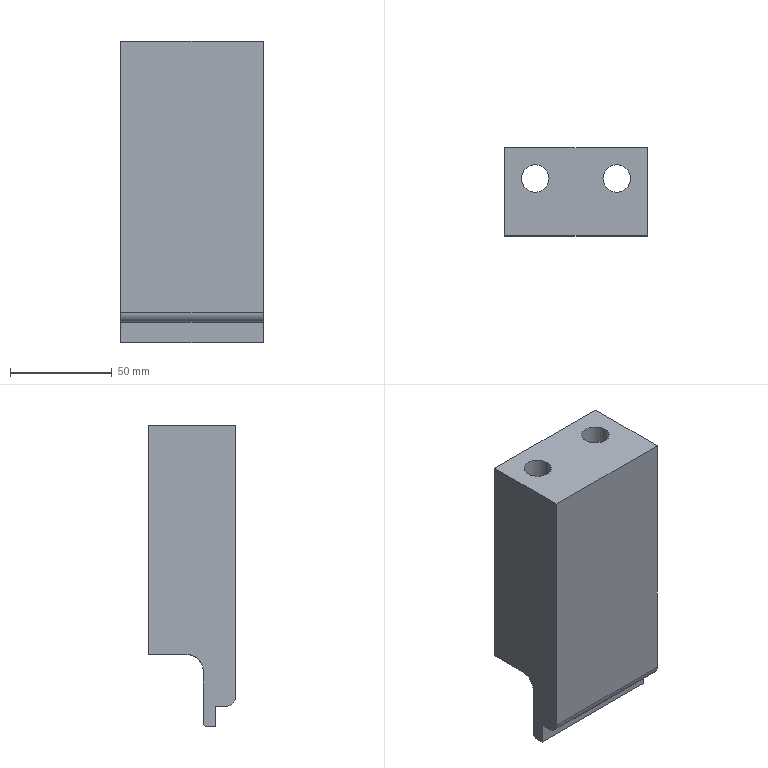Part | STEP file | lll_id3270_x_t | 1 solid | 23 faces | box 70 x 43 x 148 mm | volume 308273 mm3 | plane 13 | cylinder 9 | cone 1 | commonest cylinder face diameters 13.509 x2 20.008 x2 4 x1 10 x1 10.505 x1 14 x1
STEP:
#1=CARTESIAN_POINT('',(1635.83,35.,12.5));
#2=VERTEX_POINT('',#1);
#3=CARTESIAN_POINT('',(1654.17,35.,12.5));
#4=VERTEX_POINT('',#3);
#5=CARTESIAN_POINT('',(1645.,39.,12.5));
#6=DIRECTION('',(0.,0.,-1.));
#7=DIRECTION('',(0.,1.,0.));
#8=AXIS2_PLACEMENT_3D('',#5,#6,#7);
#9=CIRCLE('',#8,10.004);
#10=EDGE_CURVE('',#2,#4,#9,.T.);
#11=ORIENTED_EDGE('',*,*,#10,.F.);
#12=CARTESIAN_POINT('',(1625.,35.,12.5));
#13=VERTEX_POINT('',#12);
#14=CARTESIAN_POINT('',(12283.883,35.,12.5));
#15=DIRECTION('',(-1.,0.,0.));
#16=VECTOR('',#15,1.);
#17=LINE('',#14,#16);
#18=EDGE_CURVE('',#2,#13,#17,.T.);
#19=ORIENTED_EDGE('',*,*,#18,.T.);
#20=CARTESIAN_POINT('',(1625.,42.,12.5));
#21=DIRECTION('',(0.,0.,1.));
#22=DIRECTION('',(1.,0.,0.));
#23=AXIS2_PLACEMENT_3D('',#20,#21,#22);
#24=CIRCLE('',#23,7.);
#25=EDGE_CURVE('',#13,#13,#24,.T.);
#26=ORIENTED_EDGE('',*,*,#25,.T.);
#27=CARTESIAN_POINT('',(1614.17,35.,12.5));
#28=VERTEX_POINT('',#27);
#29=CARTESIAN_POINT('',(12283.883,35.,12.5));
#30=DIRECTION('',(-1.,0.,0.));
#31=VECTOR('',#30,1.);
#32=LINE('',#29,#31);
#33=EDGE_CURVE('',#13,#28,#32,.T.);
#34=ORIENTED_EDGE('',*,*,#33,.T.);
#35=CARTESIAN_POINT('',(1595.83,35.,12.5));
#36=VERTEX_POINT('',#35);
#37=CARTESIAN_POINT('',(1605.,39.,12.5));
#38=DIRECTION('',(0.,0.,1.));
#39=DIRECTION('',(0.,1.,0.));
#40=AXIS2_PLACEMENT_3D('',#37,#38,#39);
#41=CIRCLE('',#40,10.004);
#42=EDGE_CURVE('',#28,#36,#41,.T.);
#43=ORIENTED_EDGE('',*,*,#42,.T.);
#44=CARTESIAN_POINT('',(1590.,35.,12.5));
#45=VERTEX_POINT('',#44);
#46=CARTESIAN_POINT('',(12283.883,35.,12.5));
#47=DIRECTION('',(-1.,0.,0.));
#48=VECTOR('',#47,1.);
#49=LINE('',#46,#48);
#50=EDGE_CURVE('',#36,#45,#49,.T.);
#51=ORIENTED_EDGE('',*,*,#50,.T.);
#52=CARTESIAN_POINT('',(1590.,54.,12.5));
#53=VERTEX_POINT('',#52);
#54=CARTESIAN_POINT('',(1590.,13712.786,12.5));
#55=DIRECTION('',(0.,-1.,0.));
#56=VECTOR('',#55,1.);
#57=LINE('',#54,#56);
#58=EDGE_CURVE('',#53,#45,#57,.T.);
#59=ORIENTED_EDGE('',*,*,#58,.F.);
#60=CARTESIAN_POINT('',(1660.,54.,12.5));
#61=VERTEX_POINT('',#60);
#62=CARTESIAN_POINT('',(12283.883,54.,12.5));
#63=DIRECTION('',(1.,0.,0.));
#64=VECTOR('',#63,1.);
#65=LINE('',#62,#64);
#66=EDGE_CURVE('',#53,#61,#65,.T.);
#67=ORIENTED_EDGE('',*,*,#66,.T.);
#68=CARTESIAN_POINT('',(1660.,35.,12.5));
#69=VERTEX_POINT('',#68);
#70=CARTESIAN_POINT('',(1660.,11.,12.5));
#71=DIRECTION('',(0.,-1.,0.));
#72=VECTOR('',#71,1.);
#73=LINE('',#70,#72);
#74=EDGE_CURVE('',#61,#69,#73,.T.);
#75=ORIENTED_EDGE('',*,*,#74,.T.);
#76=CARTESIAN_POINT('',(12283.883,35.,12.5));
#77=DIRECTION('',(-1.,0.,0.));
#78=VECTOR('',#77,1.);
#79=LINE('',#76,#78);
#80=EDGE_CURVE('',#69,#4,#79,.T.);
#81=ORIENTED_EDGE('',*,*,#80,.T.);
#82=EDGE_LOOP('',(#11,#19,#26,#34,#43,#51,#59,#67,#75,#81));
#83=FACE_OUTER_BOUND('',#82,.T.);
#84=CARTESIAN_POINT('',(12283.883,13712.786,12.5));
#85=DIRECTION('',(0.,0.,-1.));
#86=DIRECTION('',(1.,0.,0.));
#87=AXIS2_PLACEMENT_3D('',#84,#85,#86);
#88=PLANE('',#87);
#89=ADVANCED_FACE('',(#83),#88,.T.);
#90=CARTESIAN_POINT('',(1654.17,35.,12.5));
#91=CARTESIAN_POINT('',(1653.362,33.148,12.5));
#92=CARTESIAN_POINT('',(1652.053,31.658,11.873));
#93=CARTESIAN_POINT('',(1648.893,29.593,10.524));
#94=CARTESIAN_POINT('',(1647.021,28.997,9.788));
#95=CARTESIAN_POINT('',(1642.985,28.995,9.786));
#96=CARTESIAN_POINT('',(1641.109,29.592,10.523));
#97=CARTESIAN_POINT('',(1637.948,31.657,11.872));
#98=CARTESIAN_POINT('',(1636.639,33.147,12.5));
#99=CARTESIAN_POINT('',(1635.83,35.,12.5));
#100=B_SPLINE_CURVE_WITH_KNOTS('',3,(#90,#91,#92,#93,#94,#95,#96,#97,#98,#99),.UNSPECIFIED.,.F.,.F.,(4,2,2,2,4),(0.,0.25,0.5,0.75,1.),.UNSPECIFIED.);
#101=EDGE_CURVE('',#4,#2,#100,.T.);
#102=ORIENTED_EDGE('',*,*,#101,.F.);
#103=ORIENTED_EDGE('',*,*,#80,.F.);
#104=CARTESIAN_POINT('',(1660.,27.,4.5));
#105=VERTEX_POINT('',#104);
#106=CARTESIAN_POINT('',(1660.,35.,4.5));
#107=DIRECTION('',(-1.,0.,0.));
#108=DIRECTION('',(0.,0.,-1.));
#109=AXIS2_PLACEMENT_3D('',#106,#107,#108);
#110=CIRCLE('',#109,8.);
#111=EDGE_CURVE('',#105,#69,#110,.T.);
#112=ORIENTED_EDGE('',*,*,#111,.F.);
#113=CARTESIAN_POINT('',(1590.,27.,4.5));
#114=VERTEX_POINT('',#113);
#115=CARTESIAN_POINT('',(1660.,27.,4.5));
#116=DIRECTION('',(1.,0.,0.));
#117=VECTOR('',#116,1.);
#118=LINE('',#115,#117);
#119=EDGE_CURVE('',#114,#105,#118,.T.);
#120=ORIENTED_EDGE('',*,*,#119,.F.);
#121=CARTESIAN_POINT('',(1590.,35.,4.5));
#122=DIRECTION('',(1.,0.,0.));
#123=DIRECTION('',(0.,0.,1.));
#124=AXIS2_PLACEMENT_3D('',#121,#122,#123);
#125=CIRCLE('',#124,8.);
#126=EDGE_CURVE('',#45,#114,#125,.T.);
#127=ORIENTED_EDGE('',*,*,#126,.F.);
#128=ORIENTED_EDGE('',*,*,#50,.F.);
#129=CARTESIAN_POINT('',(1595.83,35.,12.5));
#130=CARTESIAN_POINT('',(1596.638,33.148,12.5));
#131=CARTESIAN_POINT('',(1597.947,31.658,11.873));
#132=CARTESIAN_POINT('',(1601.107,29.593,10.524));
#133=CARTESIAN_POINT('',(1602.979,28.997,9.788));
#134=CARTESIAN_POINT('',(1607.015,28.995,9.786));
#135=CARTESIAN_POINT('',(1608.891,29.592,10.523));
#136=CARTESIAN_POINT('',(1612.052,31.657,11.872));
#137=CARTESIAN_POINT('',(1613.361,33.147,12.5));
#138=CARTESIAN_POINT('',(1614.17,35.,12.5));
#139=B_SPLINE_CURVE_WITH_KNOTS('',3,(#129,#130,#131,#132,#133,#134,#135,#136,#137,#138),.UNSPECIFIED.,.F.,.F.,(4,2,2,2,4),(0.,0.25,0.5,0.75,1.),.UNSPECIFIED.);
#140=EDGE_CURVE('',#36,#28,#139,.T.);
#141=ORIENTED_EDGE('',*,*,#140,.T.);
#142=ORIENTED_EDGE('',*,*,#33,.F.);
#143=ORIENTED_EDGE('',*,*,#18,.F.);
#144=EDGE_LOOP('',(#102,#103,#112,#120,#127,#128,#141,#142,#143));
#145=FACE_OUTER_BOUND('',#144,.T.);
#146=CARTESIAN_POINT('',(1660.,35.,4.5));
#147=DIRECTION('',(-1.,0.,0.));
#148=DIRECTION('',(0.,0.,1.));
#149=AXIS2_PLACEMENT_3D('',#146,#147,#148);
#150=CYLINDRICAL_SURFACE('',#149,8.);
#151=ADVANCED_FACE('',(#145),#150,.F.);
#152=CARTESIAN_POINT('',(1590.,25.,-23.));
#153=VERTEX_POINT('',#152);
#154=CARTESIAN_POINT('',(1590.,21.,-23.));
#155=VERTEX_POINT('',#154);
#156=CARTESIAN_POINT('',(1590.,30.,-23.));
#157=DIRECTION('',(0.,-1.,0.));
#158=VECTOR('',#157,1.);
#159=LINE('',#156,#158);
#160=EDGE_CURVE('',#153,#155,#159,.T.);
#161=ORIENTED_EDGE('',*,*,#160,.T.);
#162=CARTESIAN_POINT('',(1590.,21.,-13.));
#163=VERTEX_POINT('',#162);
#164=CARTESIAN_POINT('',(1590.,21.,82.));
#165=DIRECTION('',(0.,0.,1.));
#166=VECTOR('',#165,1.);
#167=LINE('',#164,#166);
#168=EDGE_CURVE('',#155,#163,#167,.T.);
#169=ORIENTED_EDGE('',*,*,#168,.T.);
#170=CARTESIAN_POINT('',(1590.,16.,-13.));
#171=VERTEX_POINT('',#170);
#172=CARTESIAN_POINT('',(1590.,1.5,-13.));
#173=DIRECTION('',(0.,-1.,0.));
#174=VECTOR('',#173,1.);
#175=LINE('',#172,#174);
#176=EDGE_CURVE('',#163,#171,#175,.T.);
#177=ORIENTED_EDGE('',*,*,#176,.T.);
#178=CARTESIAN_POINT('',(1590.,11.,-8.));
#179=VERTEX_POINT('',#178);
#180=CARTESIAN_POINT('',(1590.,16.,-8.));
#181=DIRECTION('',(1.,0.,0.));
#182=DIRECTION('',(0.,0.,1.));
#183=AXIS2_PLACEMENT_3D('',#180,#181,#182);
#184=CIRCLE('',#183,5.);
#185=EDGE_CURVE('',#179,#171,#184,.T.);
#186=ORIENTED_EDGE('',*,*,#185,.F.);
#187=CARTESIAN_POINT('',(1590.,11.,125.));
#188=VERTEX_POINT('',#187);
#189=CARTESIAN_POINT('',(1590.,11.,87.));
#190=DIRECTION('',(0.,0.,-1.));
#191=VECTOR('',#190,1.);
#192=LINE('',#189,#191);
#193=EDGE_CURVE('',#188,#179,#192,.T.);
#194=ORIENTED_EDGE('',*,*,#193,.F.);
#195=CARTESIAN_POINT('',(1590.,54.,125.));
#196=VERTEX_POINT('',#195);
#197=CARTESIAN_POINT('',(1590.,235.,125.));
#198=DIRECTION('',(0.,-1.,0.));
#199=VECTOR('',#198,1.);
#200=LINE('',#197,#199);
#201=EDGE_CURVE('',#196,#188,#200,.T.);
#202=ORIENTED_EDGE('',*,*,#201,.F.);
#203=CARTESIAN_POINT('',(1590.,54.,87.));
#204=DIRECTION('',(0.,0.,-1.));
#205=VECTOR('',#204,1.);
#206=LINE('',#203,#205);
#207=EDGE_CURVE('',#196,#53,#206,.T.);
#208=ORIENTED_EDGE('',*,*,#207,.T.);
#209=ORIENTED_EDGE('',*,*,#58,.T.);
#210=ORIENTED_EDGE('',*,*,#126,.T.);
#211=CARTESIAN_POINT('',(1590.,27.,-21.));
#212=VERTEX_POINT('',#211);
#213=CARTESIAN_POINT('',(1590.,27.,87.));
#214=DIRECTION('',(0.,0.,-1.));
#215=VECTOR('',#214,1.);
#216=LINE('',#213,#215);
#217=EDGE_CURVE('',#114,#212,#216,.T.);
#218=ORIENTED_EDGE('',*,*,#217,.T.);
#219=CARTESIAN_POINT('',(1590.,25.,-21.));
#220=DIRECTION('',(1.,0.,0.));
#221=DIRECTION('',(0.,0.,1.));
#222=AXIS2_PLACEMENT_3D('',#219,#220,#221);
#223=CIRCLE('',#222,2.);
#224=EDGE_CURVE('',#153,#212,#223,.T.);
#225=ORIENTED_EDGE('',*,*,#224,.F.);
#226=EDGE_LOOP('',(#161,#169,#177,#186,#194,#202,#208,#209,#210,#218,#225));
#227=FACE_OUTER_BOUND('',#226,.T.);
#228=CARTESIAN_POINT('',(1590.,30.,87.));
#229=DIRECTION('',(-1.,0.,0.));
#230=DIRECTION('',(0.,0.,1.));
#231=AXIS2_PLACEMENT_3D('',#228,#229,#230);
#232=PLANE('',#231);
#233=ADVANCED_FACE('',(#227),#232,.T.);
#234=CARTESIAN_POINT('',(1660.,11.,125.));
#235=VERTEX_POINT('',#234);
#236=CARTESIAN_POINT('',(1660.,11.,-8.));
#237=VERTEX_POINT('',#236);
#238=CARTESIAN_POINT('',(1660.,11.,87.));
#239=DIRECTION('',(0.,0.,-1.));
#240=VECTOR('',#239,1.);
#241=LINE('',#238,#240);
#242=EDGE_CURVE('',#235,#237,#241,.T.);
#243=ORIENTED_EDGE('',*,*,#242,.F.);
#244=CARTESIAN_POINT('',(2930.,11.,125.));
#245=DIRECTION('',(1.,0.,0.));
#246=VECTOR('',#245,1.);
#247=LINE('',#244,#246);
#248=EDGE_CURVE('',#188,#235,#247,.T.);
#249=ORIENTED_EDGE('',*,*,#248,.F.);
#250=ORIENTED_EDGE('',*,*,#193,.T.);
#251=CARTESIAN_POINT('',(1590.,11.,-8.));
#252=DIRECTION('',(-1.,0.,0.));
#253=VECTOR('',#252,1.);
#254=LINE('',#251,#253);
#255=EDGE_CURVE('',#237,#179,#254,.T.);
#256=ORIENTED_EDGE('',*,*,#255,.F.);
#257=EDGE_LOOP('',(#243,#249,#250,#256));
#258=FACE_OUTER_BOUND('',#257,.T.);
#259=CARTESIAN_POINT('',(1590.,11.,87.));
#260=DIRECTION('',(0.,-1.,0.));
#261=DIRECTION('',(0.,0.,1.));
#262=AXIS2_PLACEMENT_3D('',#259,#260,#261);
#263=PLANE('',#262);
#264=ADVANCED_FACE('',(#258),#263,.T.);
#265=CARTESIAN_POINT('',(1660.,54.,125.));
#266=VERTEX_POINT('',#265);
#267=CARTESIAN_POINT('',(1660.,235.,125.));
#268=DIRECTION('',(0.,1.,0.));
#269=VECTOR('',#268,1.);
#270=LINE('',#267,#269);
#271=EDGE_CURVE('',#235,#266,#270,.T.);
#272=ORIENTED_EDGE('',*,*,#271,.F.);
#273=ORIENTED_EDGE('',*,*,#242,.T.);
#274=CARTESIAN_POINT('',(1660.,16.,-13.));
#275=VERTEX_POINT('',#274);
#276=CARTESIAN_POINT('',(1660.,16.,-8.));
#277=DIRECTION('',(-1.,0.,0.));
#278=DIRECTION('',(0.,0.,-1.));
#279=AXIS2_PLACEMENT_3D('',#276,#277,#278);
#280=CIRCLE('',#279,5.);
#281=EDGE_CURVE('',#275,#237,#280,.T.);
#282=ORIENTED_EDGE('',*,*,#281,.F.);
#283=CARTESIAN_POINT('',(1660.,21.,-13.));
#284=VERTEX_POINT('',#283);
#285=CARTESIAN_POINT('',(1660.,1.5,-13.));
#286=DIRECTION('',(0.,1.,0.));
#287=VECTOR('',#286,1.);
#288=LINE('',#285,#287);
#289=EDGE_CURVE('',#275,#284,#288,.T.);
#290=ORIENTED_EDGE('',*,*,#289,.T.);
#291=CARTESIAN_POINT('',(1660.,21.,-23.));
#292=VERTEX_POINT('',#291);
#293=CARTESIAN_POINT('',(1660.,21.,82.));
#294=DIRECTION('',(0.,0.,-1.));
#295=VECTOR('',#294,1.);
#296=LINE('',#293,#295);
#297=EDGE_CURVE('',#284,#292,#296,.T.);
#298=ORIENTED_EDGE('',*,*,#297,.T.);
#299=CARTESIAN_POINT('',(1660.,25.,-23.));
#300=VERTEX_POINT('',#299);
#301=CARTESIAN_POINT('',(1660.,11.,-23.));
#302=DIRECTION('',(0.,1.,0.));
#303=VECTOR('',#302,1.);
#304=LINE('',#301,#303);
#305=EDGE_CURVE('',#292,#300,#304,.T.);
#306=ORIENTED_EDGE('',*,*,#305,.T.);
#307=CARTESIAN_POINT('',(1660.,27.,-21.));
#308=VERTEX_POINT('',#307);
#309=CARTESIAN_POINT('',(1660.,25.,-21.));
#310=DIRECTION('',(-1.,0.,0.));
#311=DIRECTION('',(0.,0.,-1.));
#312=AXIS2_PLACEMENT_3D('',#309,#310,#311);
#313=CIRCLE('',#312,2.);
#314=EDGE_CURVE('',#308,#300,#313,.T.);
#315=ORIENTED_EDGE('',*,*,#314,.F.);
#316=CARTESIAN_POINT('',(1660.,27.,87.));
#317=DIRECTION('',(0.,0.,-1.));
#318=VECTOR('',#317,1.);
#319=LINE('',#316,#318);
#320=EDGE_CURVE('',#105,#308,#319,.T.);
#321=ORIENTED_EDGE('',*,*,#320,.F.);
#322=ORIENTED_EDGE('',*,*,#111,.T.);
#323=ORIENTED_EDGE('',*,*,#74,.F.);
#324=CARTESIAN_POINT('',(1660.,54.,-650.));
#325=DIRECTION('',(0.,0.,-1.));
#326=VECTOR('',#325,1.);
#327=LINE('',#324,#326);
#328=EDGE_CURVE('',#266,#61,#327,.T.);
#329=ORIENTED_EDGE('',*,*,#328,.F.);
#330=EDGE_LOOP('',(#272,#273,#282,#290,#298,#306,#315,#321,#322,#323,#329));
#331=FACE_OUTER_BOUND('',#330,.T.);
#332=CARTESIAN_POINT('',(1660.,11.,87.));
#333=DIRECTION('',(1.,0.,0.));
#334=DIRECTION('',(0.,0.,-1.));
#335=AXIS2_PLACEMENT_3D('',#332,#333,#334);
#336=PLANE('',#335);
#337=ADVANCED_FACE('',(#331),#336,.T.);
#338=CARTESIAN_POINT('',(1598.245,39.,125.));
#339=VERTEX_POINT('',#338);
#340=CARTESIAN_POINT('',(1605.,39.,125.));
#341=DIRECTION('',(0.,0.,1.));
#342=DIRECTION('',(-1.,0.,0.));
#343=AXIS2_PLACEMENT_3D('',#340,#341,#342);
#344=CIRCLE('',#343,6.755);
#345=EDGE_CURVE('',#339,#339,#344,.T.);
#346=ORIENTED_EDGE('',*,*,#345,.F.);
#347=EDGE_LOOP('',(#346));
#348=FACE_BOUND('',#347,.T.);
#349=CARTESIAN_POINT('',(1638.245,39.,125.));
#350=VERTEX_POINT('',#349);
#351=CARTESIAN_POINT('',(1645.,39.,125.));
#352=DIRECTION('',(0.,0.,1.));
#353=DIRECTION('',(-1.,0.,0.));
#354=AXIS2_PLACEMENT_3D('',#351,#352,#353);
#355=CIRCLE('',#354,6.755);
#356=EDGE_CURVE('',#350,#350,#355,.T.);
#357=ORIENTED_EDGE('',*,*,#356,.F.);
#358=EDGE_LOOP('',(#357));
#359=FACE_BOUND('',#358,.T.);
#360=ORIENTED_EDGE('',*,*,#201,.T.);
#361=ORIENTED_EDGE('',*,*,#248,.T.);
#362=ORIENTED_EDGE('',*,*,#271,.T.);
#363=CARTESIAN_POINT('',(6303.751,54.,125.));
#364=DIRECTION('',(-1.,0.,0.));
#365=VECTOR('',#364,1.);
#366=LINE('',#363,#365);
#367=EDGE_CURVE('',#266,#196,#366,.T.);
#368=ORIENTED_EDGE('',*,*,#367,.T.);
#369=EDGE_LOOP('',(#360,#361,#362,#368));
#370=FACE_BOUND('',#369,.T.);
#371=CARTESIAN_POINT('',(2930.,235.,125.));
#372=DIRECTION('',(0.,0.,-1.));
#373=DIRECTION('',(-1.,0.,0.));
#374=AXIS2_PLACEMENT_3D('',#371,#372,#373);
#375=PLANE('',#374);
#376=ADVANCED_FACE('',(#348,#359,#370),#375,.F.);
#377=ORIENTED_EDGE('',*,*,#176,.F.);
#378=CARTESIAN_POINT('',(6303.751,21.,-13.));
#379=DIRECTION('',(1.,0.,0.));
#380=VECTOR('',#379,1.);
#381=LINE('',#378,#380);
#382=EDGE_CURVE('',#163,#284,#381,.T.);
#383=ORIENTED_EDGE('',*,*,#382,.T.);
#384=ORIENTED_EDGE('',*,*,#289,.F.);
#385=CARTESIAN_POINT('',(6303.751,16.,-13.));
#386=DIRECTION('',(1.,0.,0.));
#387=VECTOR('',#386,1.);
#388=LINE('',#385,#387);
#389=EDGE_CURVE('',#171,#275,#388,.T.);
#390=ORIENTED_EDGE('',*,*,#389,.F.);
#391=EDGE_LOOP('',(#377,#383,#384,#390));
#392=FACE_OUTER_BOUND('',#391,.T.);
#393=CARTESIAN_POINT('',(6303.751,1.5,-13.));
#394=DIRECTION('',(0.,0.,-1.));
#395=DIRECTION('',(-1.,0.,0.));
#396=AXIS2_PLACEMENT_3D('',#393,#394,#395);
#397=PLANE('',#396);
#398=ADVANCED_FACE('',(#392),#397,.T.);
#399=ORIENTED_EDGE('',*,*,#185,.T.);
#400=ORIENTED_EDGE('',*,*,#389,.T.);
#401=ORIENTED_EDGE('',*,*,#281,.T.);
#402=ORIENTED_EDGE('',*,*,#255,.T.);
#403=EDGE_LOOP('',(#399,#400,#401,#402));
#404=FACE_OUTER_BOUND('',#403,.T.);
#405=CARTESIAN_POINT('',(6303.751,16.,-8.));
#406=DIRECTION('',(1.,0.,0.));
#407=DIRECTION('',(0.,0.,-1.));
#408=AXIS2_PLACEMENT_3D('',#405,#406,#407);
#409=CYLINDRICAL_SURFACE('',#408,5.);
#410=ADVANCED_FACE('',(#404),#409,.T.);
#411=ORIENTED_EDGE('',*,*,#168,.F.);
#412=CARTESIAN_POINT('',(6303.751,21.,-23.));
#413=DIRECTION('',(-1.,0.,0.));
#414=VECTOR('',#413,1.);
#415=LINE('',#412,#414);
#416=EDGE_CURVE('',#292,#155,#415,.T.);
#417=ORIENTED_EDGE('',*,*,#416,.F.);
#418=ORIENTED_EDGE('',*,*,#297,.F.);
#419=ORIENTED_EDGE('',*,*,#382,.F.);
#420=EDGE_LOOP('',(#411,#417,#418,#419));
#421=FACE_OUTER_BOUND('',#420,.T.);
#422=CARTESIAN_POINT('',(1625.,21.,32.));
#423=DIRECTION('',(0.,-1.,0.));
#424=DIRECTION('',(0.,0.,1.));
#425=AXIS2_PLACEMENT_3D('',#422,#423,#424);
#426=PLANE('',#425);
#427=ADVANCED_FACE('',(#421),#426,.T.);
#428=ORIENTED_EDGE('',*,*,#217,.F.);
#429=ORIENTED_EDGE('',*,*,#119,.T.);
#430=ORIENTED_EDGE('',*,*,#320,.T.);
#431=CARTESIAN_POINT('',(6303.751,27.,-21.));
#432=DIRECTION('',(1.,0.,0.));
#433=VECTOR('',#432,1.);
#434=LINE('',#431,#433);
#435=EDGE_CURVE('',#212,#308,#434,.T.);
#436=ORIENTED_EDGE('',*,*,#435,.F.);
#437=EDGE_LOOP('',(#428,#429,#430,#436));
#438=FACE_OUTER_BOUND('',#437,.T.);
#439=CARTESIAN_POINT('',(1660.,27.,87.));
#440=DIRECTION('',(0.,1.,0.));
#441=DIRECTION('',(0.,0.,-1.));
#442=AXIS2_PLACEMENT_3D('',#439,#440,#441);
#443=PLANE('',#442);
#444=ADVANCED_FACE('',(#438),#443,.T.);
#445=ORIENTED_EDGE('',*,*,#305,.F.);
#446=ORIENTED_EDGE('',*,*,#416,.T.);
#447=ORIENTED_EDGE('',*,*,#160,.F.);
#448=CARTESIAN_POINT('',(6303.751,25.,-23.));
#449=DIRECTION('',(-1.,0.,0.));
#450=VECTOR('',#449,1.);
#451=LINE('',#448,#450);
#452=EDGE_CURVE('',#300,#153,#451,.T.);
#453=ORIENTED_EDGE('',*,*,#452,.F.);
#454=EDGE_LOOP('',(#445,#446,#447,#453));
#455=FACE_OUTER_BOUND('',#454,.T.);
#456=CARTESIAN_POINT('',(6303.751,1.5,-23.));
#457=DIRECTION('',(0.,0.,-1.));
#458=DIRECTION('',(-1.,0.,0.));
#459=AXIS2_PLACEMENT_3D('',#456,#457,#458);
#460=PLANE('',#459);
#461=ADVANCED_FACE('',(#455),#460,.T.);
#462=ORIENTED_EDGE('',*,*,#314,.T.);
#463=ORIENTED_EDGE('',*,*,#452,.T.);
#464=ORIENTED_EDGE('',*,*,#224,.T.);
#465=ORIENTED_EDGE('',*,*,#435,.T.);
#466=EDGE_LOOP('',(#462,#463,#464,#465));
#467=FACE_OUTER_BOUND('',#466,.T.);
#468=CARTESIAN_POINT('',(6303.751,25.,-21.));
#469=DIRECTION('',(-1.,0.,0.));
#470=DIRECTION('',(0.,0.,1.));
#471=AXIS2_PLACEMENT_3D('',#468,#469,#470);
#472=CYLINDRICAL_SURFACE('',#471,2.);
#473=ADVANCED_FACE('',(#467),#472,.T.);
#474=ORIENTED_EDGE('',*,*,#66,.F.);
#475=ORIENTED_EDGE('',*,*,#207,.F.);
#476=ORIENTED_EDGE('',*,*,#367,.F.);
#477=ORIENTED_EDGE('',*,*,#328,.T.);
#478=EDGE_LOOP('',(#474,#475,#476,#477));
#479=FACE_OUTER_BOUND('',#478,.T.);
#480=CARTESIAN_POINT('',(6303.751,54.,-650.));
#481=DIRECTION('',(0.,-1.,0.));
#482=DIRECTION('',(0.,0.,1.));
#483=AXIS2_PLACEMENT_3D('',#480,#481,#482);
#484=PLANE('',#483);
#485=ADVANCED_FACE('',(#479),#484,.F.);
#486=CARTESIAN_POINT('',(1632.,42.,17.5));
#487=VERTEX_POINT('',#486);
#488=CARTESIAN_POINT('',(1625.,42.,17.5));
#489=DIRECTION('',(0.,0.,1.));
#490=DIRECTION('',(1.,0.,0.));
#491=AXIS2_PLACEMENT_3D('',#488,#489,#490);
#492=CIRCLE('',#491,7.);
#493=EDGE_CURVE('',#487,#487,#492,.T.);
#494=ORIENTED_EDGE('',*,*,#493,.F.);
#495=EDGE_LOOP('',(#494));
#496=FACE_BOUND('',#495,.T.);
#497=CARTESIAN_POINT('',(1625.,36.747,17.5));
#498=VERTEX_POINT('',#497);
#499=CARTESIAN_POINT('',(1625.,42.,17.5));
#500=DIRECTION('',(0.,0.,-1.));
#501=DIRECTION('',(0.,-1.,0.));
#502=AXIS2_PLACEMENT_3D('',#499,#500,#501);
#503=CIRCLE('',#502,5.253);
#504=EDGE_CURVE('',#498,#498,#503,.T.);
#505=ORIENTED_EDGE('',*,*,#504,.F.);
#506=EDGE_LOOP('',(#505));
#507=FACE_BOUND('',#506,.T.);
#508=CARTESIAN_POINT('',(1625.,42.,17.5));
#509=DIRECTION('',(0.,0.,1.));
#510=DIRECTION('',(0.,-1.,0.));
#511=AXIS2_PLACEMENT_3D('',#508,#509,#510);
#512=PLANE('',#511);
#513=ADVANCED_FACE('',(#496,#507),#512,.F.);
#514=ORIENTED_EDGE('',*,*,#493,.T.);
#515=EDGE_LOOP('',(#514));
#516=FACE_BOUND('',#515,.T.);
#517=ORIENTED_EDGE('',*,*,#25,.F.);
#518=EDGE_LOOP('',(#517));
#519=FACE_BOUND('',#518,.T.);
#520=CARTESIAN_POINT('',(1625.,42.,12.5));
#521=DIRECTION('',(0.,0.,1.));
#522=DIRECTION('',(1.,0.,0.));
#523=AXIS2_PLACEMENT_3D('',#520,#521,#522);
#524=CYLINDRICAL_SURFACE('',#523,7.);
#525=ADVANCED_FACE('',(#516,#519),#524,.F.);
#526=CARTESIAN_POINT('',(1625.,42.,47.506));
#527=VERTEX_POINT('',#526);
#528=VERTEX_LOOP('',#527);
#529=FACE_BOUND('',#528,.T.);
#530=CARTESIAN_POINT('',(1625.,47.252,42.253));
#531=VERTEX_POINT('',#530);
#532=CARTESIAN_POINT('',(1625.,42.,42.253));
#533=DIRECTION('',(0.,0.,-1.));
#534=DIRECTION('',(0.,1.,0.));
#535=AXIS2_PLACEMENT_3D('',#532,#533,#534);
#536=CIRCLE('',#535,5.253);
#537=EDGE_CURVE('',#531,#531,#536,.T.);
#538=ORIENTED_EDGE('',*,*,#537,.T.);
#539=EDGE_LOOP('',(#538));
#540=FACE_BOUND('',#539,.T.);
#541=CARTESIAN_POINT('',(1625.,42.,42.253));
#542=DIRECTION('',(0.,0.,-1.));
#543=DIRECTION('',(0.,-1.,0.));
#544=AXIS2_PLACEMENT_3D('',#541,#542,#543);
#545=CONICAL_SURFACE('',#544,5.253,45.);
#546=ADVANCED_FACE('',(#529,#540),#545,.F.);
#547=ORIENTED_EDGE('',*,*,#504,.T.);
#548=EDGE_LOOP('',(#547));
#549=FACE_BOUND('',#548,.T.);
#550=ORIENTED_EDGE('',*,*,#537,.F.);
#551=EDGE_LOOP('',(#550));
#552=FACE_BOUND('',#551,.T.);
#553=CARTESIAN_POINT('',(1625.,42.,7.5));
#554=DIRECTION('',(0.,0.,1.));
#555=DIRECTION('',(1.,0.,0.));
#556=AXIS2_PLACEMENT_3D('',#553,#554,#555);
#557=CYLINDRICAL_SURFACE('',#556,5.253);
#558=ADVANCED_FACE('',(#549,#552),#557,.F.);
#559=CARTESIAN_POINT('',(1594.996,39.,95.));
#560=VERTEX_POINT('',#559);
#561=CARTESIAN_POINT('',(1605.,39.,95.));
#562=DIRECTION('',(0.,0.,-1.));
#563=DIRECTION('',(-1.,0.,0.));
#564=AXIS2_PLACEMENT_3D('',#561,#562,#563);
#565=CIRCLE('',#564,10.004);
#566=EDGE_CURVE('',#560,#560,#565,.T.);
#567=ORIENTED_EDGE('',*,*,#566,.F.);
#568=EDGE_LOOP('',(#567));
#569=FACE_BOUND('',#568,.T.);
#570=ORIENTED_EDGE('',*,*,#140,.F.);
#571=ORIENTED_EDGE('',*,*,#42,.F.);
#572=EDGE_LOOP('',(#570,#571));
#573=FACE_BOUND('',#572,.T.);
#574=CARTESIAN_POINT('',(1605.,39.,-1005.));
#575=DIRECTION('',(0.,0.,1.));
#576=DIRECTION('',(1.,0.,0.));
#577=AXIS2_PLACEMENT_3D('',#574,#575,#576);
#578=CYLINDRICAL_SURFACE('',#577,10.004);
#579=ADVANCED_FACE('',(#569,#573),#578,.F.);
#580=CARTESIAN_POINT('',(1598.245,39.,95.));
#581=VERTEX_POINT('',#580);
#582=CARTESIAN_POINT('',(1605.,39.,95.));
#583=DIRECTION('',(0.,0.,-1.));
#584=DIRECTION('',(-1.,0.,0.));
#585=AXIS2_PLACEMENT_3D('',#582,#583,#584);
#586=CIRCLE('',#585,6.755);
#587=EDGE_CURVE('',#581,#581,#586,.T.);
#588=ORIENTED_EDGE('',*,*,#587,.F.);
#589=EDGE_LOOP('',(#588));
#590=FACE_BOUND('',#589,.T.);
#591=ORIENTED_EDGE('',*,*,#566,.T.);
#592=EDGE_LOOP('',(#591));
#593=FACE_BOUND('',#592,.T.);
#594=CARTESIAN_POINT('',(1605.,39.,95.));
#595=DIRECTION('',(0.,0.,1.));
#596=DIRECTION('',(1.,0.,0.));
#597=AXIS2_PLACEMENT_3D('',#594,#595,#596);
#598=PLANE('',#597);
#599=ADVANCED_FACE('',(#590,#593),#598,.F.);
#600=CARTESIAN_POINT('',(1634.996,39.,95.));
#601=VERTEX_POINT('',#600);
#602=CARTESIAN_POINT('',(1645.,39.,95.));
#603=DIRECTION('',(0.,0.,1.));
#604=DIRECTION('',(-1.,0.,0.));
#605=AXIS2_PLACEMENT_3D('',#602,#603,#604);
#606=CIRCLE('',#605,10.004);
#607=EDGE_CURVE('',#601,#601,#606,.T.);
#608=ORIENTED_EDGE('',*,*,#607,.T.);
#609=EDGE_LOOP('',(#608));
#610=FACE_BOUND('',#609,.T.);
#611=ORIENTED_EDGE('',*,*,#10,.T.);
#612=ORIENTED_EDGE('',*,*,#101,.T.);
#613=EDGE_LOOP('',(#611,#612));
#614=FACE_BOUND('',#613,.T.);
#615=CARTESIAN_POINT('',(1645.,39.,-1005.));
#616=DIRECTION('',(0.,0.,1.));
#617=DIRECTION('',(1.,0.,0.));
#618=AXIS2_PLACEMENT_3D('',#615,#616,#617);
#619=CYLINDRICAL_SURFACE('',#618,10.004);
#620=ADVANCED_FACE('',(#610,#614),#619,.F.);
#621=CARTESIAN_POINT('',(1638.245,39.,95.));
#622=VERTEX_POINT('',#621);
#623=CARTESIAN_POINT('',(1645.,39.,95.));
#624=DIRECTION('',(0.,0.,-1.));
#625=DIRECTION('',(-1.,0.,0.));
#626=AXIS2_PLACEMENT_3D('',#623,#624,#625);
#627=CIRCLE('',#626,6.755);
#628=EDGE_CURVE('',#622,#622,#627,.T.);
#629=ORIENTED_EDGE('',*,*,#628,.F.);
#630=EDGE_LOOP('',(#629));
#631=FACE_BOUND('',#630,.T.);
#632=ORIENTED_EDGE('',*,*,#607,.F.);
#633=EDGE_LOOP('',(#632));
#634=FACE_BOUND('',#633,.T.);
#635=CARTESIAN_POINT('',(1645.,39.,95.));
#636=DIRECTION('',(0.,0.,-1.));
#637=DIRECTION('',(-1.,0.,0.));
#638=AXIS2_PLACEMENT_3D('',#635,#636,#637);
#639=PLANE('',#638);
#640=ADVANCED_FACE('',(#631,#634),#639,.T.);
#641=ORIENTED_EDGE('',*,*,#628,.T.);
#642=EDGE_LOOP('',(#641));
#643=FACE_BOUND('',#642,.T.);
#644=ORIENTED_EDGE('',*,*,#356,.T.);
#645=EDGE_LOOP('',(#644));
#646=FACE_BOUND('',#645,.T.);
#647=CARTESIAN_POINT('',(1645.,39.,7.5));
#648=DIRECTION('',(0.,0.,1.));
#649=DIRECTION('',(1.,0.,0.));
#650=AXIS2_PLACEMENT_3D('',#647,#648,#649);
#651=CYLINDRICAL_SURFACE('',#650,6.755);
#652=ADVANCED_FACE('',(#643,#646),#651,.F.);
#653=ORIENTED_EDGE('',*,*,#587,.T.);
#654=EDGE_LOOP('',(#653));
#655=FACE_BOUND('',#654,.T.);
#656=ORIENTED_EDGE('',*,*,#345,.T.);
#657=EDGE_LOOP('',(#656));
#658=FACE_BOUND('',#657,.T.);
#659=CARTESIAN_POINT('',(1605.,39.,7.5));
#660=DIRECTION('',(0.,0.,1.));
#661=DIRECTION('',(-1.,0.,0.));
#662=AXIS2_PLACEMENT_3D('',#659,#660,#661);
#663=CYLINDRICAL_SURFACE('',#662,6.755);
#664=ADVANCED_FACE('',(#655,#658),#663,.F.);
#665=CLOSED_SHELL('',(#89,#151,#233,#264,#337,#376,#398,#410,#427,#444,#461,#473,#485,#513,#525,#546,#558,#579,#599,#620,#640,#652,#664));
#666=MANIFOLD_SOLID_BREP('',#665);
#667=(LENGTH_UNIT()NAMED_UNIT(*)SI_UNIT(.MILLI.,.METRE.));
#668=UNCERTAINTY_MEASURE_WITH_UNIT(LENGTH_MEASURE(0.0508),#667,'','');
#669=(NAMED_UNIT(*)PLANE_ANGLE_UNIT()SI_UNIT($,.RADIAN.));
#670=PLANE_ANGLE_MEASURE_WITH_UNIT(PLANE_ANGLE_MEASURE(0.01745),#669);
#671=DIMENSIONAL_EXPONENTS(0.,0.,0.,0.,0.,0.,0.);
#672=(CONVERSION_BASED_UNIT('DEGREE',#670)NAMED_UNIT(#671)PLANE_ANGLE_UNIT());
#673=(NAMED_UNIT(*)SI_UNIT($,.STERADIAN.)SOLID_ANGLE_UNIT());
#674=(GEOMETRIC_REPRESENTATION_CONTEXT(3)GLOBAL_UNCERTAINTY_ASSIGNED_CONTEXT((#668))GLOBAL_UNIT_ASSIGNED_CONTEXT((#667,#672,#673))REPRESENTATION_CONTEXT('',''));
#675=ADVANCED_BREP_SHAPE_REPRESENTATION('',(#666),#674);